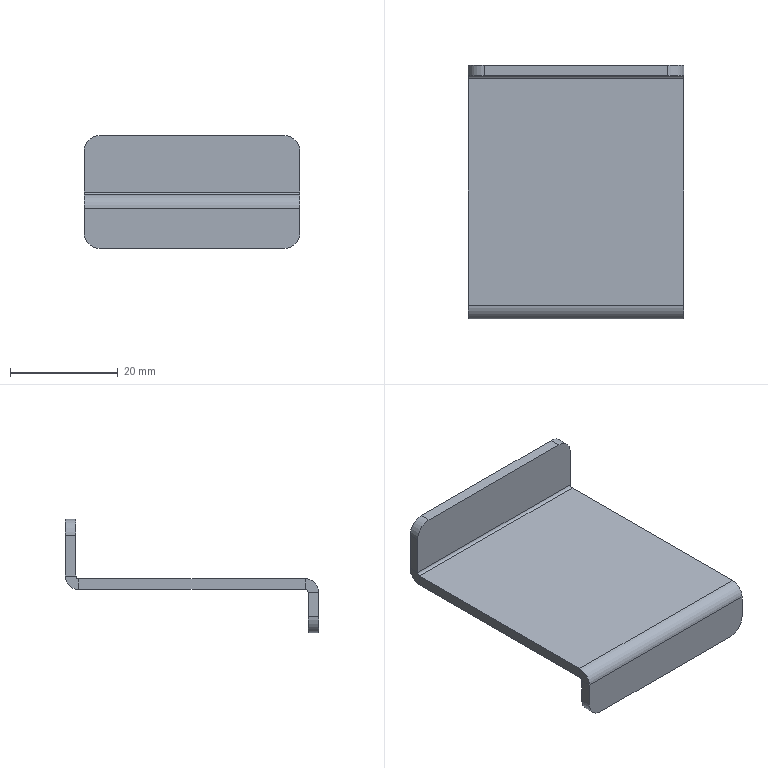Part | SolidWorks | features BaseBody 1 | 1 solid | 26 faces | box 40 x 47 x 21 mm | volume 5162 mm3 | plane 18 | cylinder 8 | commonest cylinder face diameters 6 x4 1 x2 5 x2
STEP:
#1=CARTESIAN_POINT('',(17.,-23.5,-10.));
#2=VERTEX_POINT('',#1);
#3=CARTESIAN_POINT('',(20.,-23.5,-7.));
#4=VERTEX_POINT('',#3);
#5=CARTESIAN_POINT('',(17.,-23.5,-7.));
#6=DIRECTION('',(0.,-1.,0.));
#7=DIRECTION('',(0.,0.,-1.));
#8=AXIS2_PLACEMENT_3D('',#5,#6,#7);
#9=CIRCLE('',#8,3.);
#10=EDGE_CURVE('',#2,#4,#9,.T.);
#11=ORIENTED_EDGE('',*,*,#10,.F.);
#12=CARTESIAN_POINT('',(17.,-21.5,-10.));
#13=VERTEX_POINT('',#12);
#14=CARTESIAN_POINT('',(17.,-23.5,-10.));
#15=DIRECTION('',(0.,-1.,0.));
#16=VECTOR('',#15,1000.);
#17=LINE('',#14,#16);
#18=EDGE_CURVE('',#13,#2,#17,.T.);
#19=ORIENTED_EDGE('',*,*,#18,.F.);
#20=CARTESIAN_POINT('',(20.,-21.5,-7.));
#21=VERTEX_POINT('',#20);
#22=CARTESIAN_POINT('',(17.,-21.5,-7.));
#23=DIRECTION('',(0.,1.,0.));
#24=DIRECTION('',(0.,0.,-1.));
#25=AXIS2_PLACEMENT_3D('',#22,#23,#24);
#26=CIRCLE('',#25,3.);
#27=EDGE_CURVE('',#21,#13,#26,.T.);
#28=ORIENTED_EDGE('',*,*,#27,.F.);
#29=CARTESIAN_POINT('',(20.,-23.5,-7.));
#30=DIRECTION('',(0.,1.,0.));
#31=VECTOR('',#30,1000.);
#32=LINE('',#29,#31);
#33=EDGE_CURVE('',#4,#21,#32,.T.);
#34=ORIENTED_EDGE('',*,*,#33,.F.);
#35=EDGE_LOOP('',(#11,#19,#28,#34));
#36=FACE_OUTER_BOUND('',#35,.T.);
#37=CARTESIAN_POINT('',(17.,-23.5,-7.));
#38=DIRECTION('',(0.,1.,0.));
#39=DIRECTION('',(0.,0.,1.));
#40=AXIS2_PLACEMENT_3D('',#37,#38,#39);
#41=CYLINDRICAL_SURFACE('',#40,3.);
#42=ADVANCED_FACE('',(#36),#41,.T.);
#43=CARTESIAN_POINT('',(-20.,-23.5,-7.));
#44=VERTEX_POINT('',#43);
#45=CARTESIAN_POINT('',(-17.,-23.5,-10.));
#46=VERTEX_POINT('',#45);
#47=CARTESIAN_POINT('',(-17.,-23.5,-7.));
#48=DIRECTION('',(0.,-1.,0.));
#49=DIRECTION('',(0.,0.,-1.));
#50=AXIS2_PLACEMENT_3D('',#47,#48,#49);
#51=CIRCLE('',#50,3.);
#52=EDGE_CURVE('',#44,#46,#51,.T.);
#53=ORIENTED_EDGE('',*,*,#52,.F.);
#54=CARTESIAN_POINT('',(-20.,-21.5,-7.));
#55=VERTEX_POINT('',#54);
#56=CARTESIAN_POINT('',(-20.,-23.5,-7.));
#57=DIRECTION('',(0.,-1.,0.));
#58=VECTOR('',#57,1000.);
#59=LINE('',#56,#58);
#60=EDGE_CURVE('',#55,#44,#59,.T.);
#61=ORIENTED_EDGE('',*,*,#60,.F.);
#62=CARTESIAN_POINT('',(-17.,-21.5,-10.));
#63=VERTEX_POINT('',#62);
#64=CARTESIAN_POINT('',(-17.,-21.5,-7.));
#65=DIRECTION('',(0.,1.,0.));
#66=DIRECTION('',(0.,0.,-1.));
#67=AXIS2_PLACEMENT_3D('',#64,#65,#66);
#68=CIRCLE('',#67,3.);
#69=EDGE_CURVE('',#63,#55,#68,.T.);
#70=ORIENTED_EDGE('',*,*,#69,.F.);
#71=CARTESIAN_POINT('',(-17.,-23.5,-10.));
#72=DIRECTION('',(0.,1.,0.));
#73=VECTOR('',#72,1000.);
#74=LINE('',#71,#73);
#75=EDGE_CURVE('',#46,#63,#74,.T.);
#76=ORIENTED_EDGE('',*,*,#75,.F.);
#77=EDGE_LOOP('',(#53,#61,#70,#76));
#78=FACE_OUTER_BOUND('',#77,.T.);
#79=CARTESIAN_POINT('',(-17.,-23.5,-7.));
#80=DIRECTION('',(0.,1.,0.));
#81=DIRECTION('',(0.,0.,1.));
#82=AXIS2_PLACEMENT_3D('',#79,#80,#81);
#83=CYLINDRICAL_SURFACE('',#82,3.);
#84=ADVANCED_FACE('',(#78),#83,.T.);
#85=CARTESIAN_POINT('',(17.,23.5,11.));
#86=VERTEX_POINT('',#85);
#87=CARTESIAN_POINT('',(20.,23.5,8.));
#88=VERTEX_POINT('',#87);
#89=CARTESIAN_POINT('',(17.,23.5,8.));
#90=DIRECTION('',(0.,1.,0.));
#91=DIRECTION('',(0.,0.,-1.));
#92=AXIS2_PLACEMENT_3D('',#89,#90,#91);
#93=CIRCLE('',#92,3.);
#94=EDGE_CURVE('',#86,#88,#93,.T.);
#95=ORIENTED_EDGE('',*,*,#94,.F.);
#96=CARTESIAN_POINT('',(17.,21.5,11.));
#97=VERTEX_POINT('',#96);
#98=CARTESIAN_POINT('',(17.,23.5,11.));
#99=DIRECTION('',(0.,1.,0.));
#100=VECTOR('',#99,1000.);
#101=LINE('',#98,#100);
#102=EDGE_CURVE('',#97,#86,#101,.T.);
#103=ORIENTED_EDGE('',*,*,#102,.F.);
#104=CARTESIAN_POINT('',(20.,21.5,8.));
#105=VERTEX_POINT('',#104);
#106=CARTESIAN_POINT('',(17.,21.5,8.));
#107=DIRECTION('',(0.,-1.,0.));
#108=DIRECTION('',(0.,0.,-1.));
#109=AXIS2_PLACEMENT_3D('',#106,#107,#108);
#110=CIRCLE('',#109,3.);
#111=EDGE_CURVE('',#105,#97,#110,.T.);
#112=ORIENTED_EDGE('',*,*,#111,.F.);
#113=CARTESIAN_POINT('',(20.,23.5,8.));
#114=DIRECTION('',(0.,-1.,0.));
#115=VECTOR('',#114,1000.);
#116=LINE('',#113,#115);
#117=EDGE_CURVE('',#88,#105,#116,.T.);
#118=ORIENTED_EDGE('',*,*,#117,.F.);
#119=EDGE_LOOP('',(#95,#103,#112,#118));
#120=FACE_OUTER_BOUND('',#119,.T.);
#121=CARTESIAN_POINT('',(17.,23.5,8.));
#122=DIRECTION('',(0.,-1.,0.));
#123=DIRECTION('',(0.,0.,-1.));
#124=AXIS2_PLACEMENT_3D('',#121,#122,#123);
#125=CYLINDRICAL_SURFACE('',#124,3.);
#126=ADVANCED_FACE('',(#120),#125,.T.);
#127=CARTESIAN_POINT('',(-20.,23.5,8.));
#128=VERTEX_POINT('',#127);
#129=CARTESIAN_POINT('',(-17.,23.5,11.));
#130=VERTEX_POINT('',#129);
#131=CARTESIAN_POINT('',(-17.,23.5,8.));
#132=DIRECTION('',(0.,1.,0.));
#133=DIRECTION('',(0.,0.,-1.));
#134=AXIS2_PLACEMENT_3D('',#131,#132,#133);
#135=CIRCLE('',#134,3.);
#136=EDGE_CURVE('',#128,#130,#135,.T.);
#137=ORIENTED_EDGE('',*,*,#136,.F.);
#138=CARTESIAN_POINT('',(-20.,21.5,8.));
#139=VERTEX_POINT('',#138);
#140=CARTESIAN_POINT('',(-20.,23.5,8.));
#141=DIRECTION('',(0.,1.,0.));
#142=VECTOR('',#141,1000.);
#143=LINE('',#140,#142);
#144=EDGE_CURVE('',#139,#128,#143,.T.);
#145=ORIENTED_EDGE('',*,*,#144,.F.);
#146=CARTESIAN_POINT('',(-17.,21.5,11.));
#147=VERTEX_POINT('',#146);
#148=CARTESIAN_POINT('',(-17.,21.5,8.));
#149=DIRECTION('',(0.,-1.,0.));
#150=DIRECTION('',(0.,0.,-1.));
#151=AXIS2_PLACEMENT_3D('',#148,#149,#150);
#152=CIRCLE('',#151,3.);
#153=EDGE_CURVE('',#147,#139,#152,.T.);
#154=ORIENTED_EDGE('',*,*,#153,.F.);
#155=CARTESIAN_POINT('',(-17.,23.5,11.));
#156=DIRECTION('',(0.,-1.,0.));
#157=VECTOR('',#156,1000.);
#158=LINE('',#155,#157);
#159=EDGE_CURVE('',#130,#147,#158,.T.);
#160=ORIENTED_EDGE('',*,*,#159,.F.);
#161=EDGE_LOOP('',(#137,#145,#154,#160));
#162=FACE_OUTER_BOUND('',#161,.T.);
#163=CARTESIAN_POINT('',(-17.,23.5,8.));
#164=DIRECTION('',(0.,-1.,0.));
#165=DIRECTION('',(0.,0.,-1.));
#166=AXIS2_PLACEMENT_3D('',#163,#164,#165);
#167=CYLINDRICAL_SURFACE('',#166,3.);
#168=ADVANCED_FACE('',(#162),#167,.T.);
#169=CARTESIAN_POINT('',(0.,23.5,11.));
#170=DIRECTION('',(1.,0.,0.));
#171=VECTOR('',#170,1000.);
#172=LINE('',#169,#171);
#173=EDGE_CURVE('',#130,#86,#172,.T.);
#174=ORIENTED_EDGE('',*,*,#173,.F.);
#175=ORIENTED_EDGE('',*,*,#159,.T.);
#176=CARTESIAN_POINT('',(20.,21.5,11.));
#177=DIRECTION('',(1.,0.,0.));
#178=VECTOR('',#177,1000.);
#179=LINE('',#176,#178);
#180=EDGE_CURVE('',#147,#97,#179,.T.);
#181=ORIENTED_EDGE('',*,*,#180,.T.);
#182=ORIENTED_EDGE('',*,*,#102,.T.);
#183=EDGE_LOOP('',(#174,#175,#181,#182));
#184=FACE_OUTER_BOUND('',#183,.T.);
#185=CARTESIAN_POINT('',(20.,23.5,11.));
#186=DIRECTION('',(0.,0.,-1.));
#187=DIRECTION('',(0.,-1.,0.));
#188=AXIS2_PLACEMENT_3D('',#185,#186,#187);
#189=PLANE('',#188);
#190=ADVANCED_FACE('',(#184),#189,.F.);
#191=ORIENTED_EDGE('',*,*,#180,.F.);
#192=ORIENTED_EDGE('',*,*,#153,.T.);
#193=CARTESIAN_POINT('',(-20.,21.5,0.5));
#194=VERTEX_POINT('',#193);
#195=CARTESIAN_POINT('',(-20.,21.5,11.));
#196=DIRECTION('',(0.,0.,1.));
#197=VECTOR('',#196,1000.);
#198=LINE('',#195,#197);
#199=EDGE_CURVE('',#194,#139,#198,.T.);
#200=ORIENTED_EDGE('',*,*,#199,.F.);
#201=CARTESIAN_POINT('',(20.,21.5,0.5));
#202=VERTEX_POINT('',#201);
#203=CARTESIAN_POINT('',(20.,21.5,0.5));
#204=DIRECTION('',(-1.,0.,0.));
#205=VECTOR('',#204,1000.);
#206=LINE('',#203,#205);
#207=EDGE_CURVE('',#202,#194,#206,.T.);
#208=ORIENTED_EDGE('',*,*,#207,.F.);
#209=CARTESIAN_POINT('',(20.,21.5,0.));
#210=DIRECTION('',(0.,0.,-1.));
#211=VECTOR('',#210,1000.);
#212=LINE('',#209,#211);
#213=EDGE_CURVE('',#105,#202,#212,.T.);
#214=ORIENTED_EDGE('',*,*,#213,.F.);
#215=ORIENTED_EDGE('',*,*,#111,.T.);
#216=EDGE_LOOP('',(#191,#192,#200,#208,#214,#215));
#217=FACE_OUTER_BOUND('',#216,.T.);
#218=CARTESIAN_POINT('',(0.,21.5,0.));
#219=DIRECTION('',(0.,-1.,0.));
#220=DIRECTION('',(-1.,0.,0.));
#221=AXIS2_PLACEMENT_3D('',#218,#219,#220);
#222=PLANE('',#221);
#223=ADVANCED_FACE('',(#217),#222,.T.);
#224=CARTESIAN_POINT('',(-20.,23.5,0.5));
#225=VERTEX_POINT('',#224);
#226=CARTESIAN_POINT('',(-20.,23.5,0.));
#227=DIRECTION('',(0.,0.,1.));
#228=VECTOR('',#227,1000.);
#229=LINE('',#226,#228);
#230=EDGE_CURVE('',#225,#128,#229,.T.);
#231=ORIENTED_EDGE('',*,*,#230,.T.);
#232=ORIENTED_EDGE('',*,*,#136,.T.);
#233=ORIENTED_EDGE('',*,*,#173,.T.);
#234=ORIENTED_EDGE('',*,*,#94,.T.);
#235=CARTESIAN_POINT('',(20.,23.5,0.5));
#236=VERTEX_POINT('',#235);
#237=CARTESIAN_POINT('',(20.,23.5,0.));
#238=DIRECTION('',(0.,0.,-1.));
#239=VECTOR('',#238,1000.);
#240=LINE('',#237,#239);
#241=EDGE_CURVE('',#88,#236,#240,.T.);
#242=ORIENTED_EDGE('',*,*,#241,.T.);
#243=CARTESIAN_POINT('',(20.,23.5,0.5));
#244=DIRECTION('',(1.,0.,0.));
#245=VECTOR('',#244,1000.);
#246=LINE('',#243,#245);
#247=EDGE_CURVE('',#225,#236,#246,.T.);
#248=ORIENTED_EDGE('',*,*,#247,.F.);
#249=EDGE_LOOP('',(#231,#232,#233,#234,#242,#248));
#250=FACE_OUTER_BOUND('',#249,.T.);
#251=CARTESIAN_POINT('',(0.,23.5,0.));
#252=DIRECTION('',(0.,-1.,0.));
#253=DIRECTION('',(-1.,0.,0.));
#254=AXIS2_PLACEMENT_3D('',#251,#252,#253);
#255=PLANE('',#254);
#256=ADVANCED_FACE('',(#250),#255,.F.);
#257=ORIENTED_EDGE('',*,*,#199,.T.);
#258=ORIENTED_EDGE('',*,*,#144,.T.);
#259=ORIENTED_EDGE('',*,*,#230,.F.);
#260=CARTESIAN_POINT('',(-20.,21.5,0.5));
#261=DIRECTION('',(0.,1.,0.));
#262=VECTOR('',#261,1000.);
#263=LINE('',#260,#262);
#264=EDGE_CURVE('',#194,#225,#263,.T.);
#265=ORIENTED_EDGE('',*,*,#264,.F.);
#266=EDGE_LOOP('',(#257,#258,#259,#265));
#267=FACE_OUTER_BOUND('',#266,.T.);
#268=CARTESIAN_POINT('',(-20.,23.5,11.));
#269=DIRECTION('',(1.,0.,0.));
#270=DIRECTION('',(0.,1.,0.));
#271=AXIS2_PLACEMENT_3D('',#268,#269,#270);
#272=PLANE('',#271);
#273=ADVANCED_FACE('',(#267),#272,.F.);
#274=ORIENTED_EDGE('',*,*,#241,.F.);
#275=ORIENTED_EDGE('',*,*,#117,.T.);
#276=ORIENTED_EDGE('',*,*,#213,.T.);
#277=CARTESIAN_POINT('',(20.,23.5,0.5));
#278=DIRECTION('',(0.,1.,0.));
#279=VECTOR('',#278,1000.);
#280=LINE('',#277,#279);
#281=EDGE_CURVE('',#202,#236,#280,.T.);
#282=ORIENTED_EDGE('',*,*,#281,.T.);
#283=EDGE_LOOP('',(#274,#275,#276,#282));
#284=FACE_OUTER_BOUND('',#283,.T.);
#285=CARTESIAN_POINT('',(20.,23.5,0.));
#286=DIRECTION('',(-1.,0.,0.));
#287=DIRECTION('',(0.,0.,1.));
#288=AXIS2_PLACEMENT_3D('',#285,#286,#287);
#289=PLANE('',#288);
#290=ADVANCED_FACE('',(#284),#289,.F.);
#291=CARTESIAN_POINT('',(-20.,21.,0.));
#292=VERTEX_POINT('',#291);
#293=CARTESIAN_POINT('',(20.,21.,0.));
#294=VERTEX_POINT('',#293);
#295=CARTESIAN_POINT('',(-20.,21.,0.));
#296=DIRECTION('',(1.,0.,0.));
#297=VECTOR('',#296,1000.);
#298=LINE('',#295,#297);
#299=EDGE_CURVE('',#292,#294,#298,.T.);
#300=ORIENTED_EDGE('',*,*,#299,.T.);
#301=CARTESIAN_POINT('',(20.,21.,0.5));
#302=DIRECTION('',(1.,0.,0.));
#303=DIRECTION('',(0.,0.,1.));
#304=AXIS2_PLACEMENT_3D('',#301,#302,#303);
#305=CIRCLE('',#304,0.5);
#306=EDGE_CURVE('',#294,#202,#305,.T.);
#307=ORIENTED_EDGE('',*,*,#306,.T.);
#308=ORIENTED_EDGE('',*,*,#207,.T.);
#309=CARTESIAN_POINT('',(-20.,21.,0.5));
#310=DIRECTION('',(-1.,0.,0.));
#311=DIRECTION('',(0.,0.,1.));
#312=AXIS2_PLACEMENT_3D('',#309,#310,#311);
#313=CIRCLE('',#312,0.5);
#314=EDGE_CURVE('',#194,#292,#313,.T.);
#315=ORIENTED_EDGE('',*,*,#314,.T.);
#316=EDGE_LOOP('',(#300,#307,#308,#315));
#317=FACE_OUTER_BOUND('',#316,.T.);
#318=CARTESIAN_POINT('',(-20.,21.,0.5));
#319=DIRECTION('',(-1.,0.,0.));
#320=DIRECTION('',(0.,1.,0.));
#321=AXIS2_PLACEMENT_3D('',#318,#319,#320);
#322=CYLINDRICAL_SURFACE('',#321,0.5);
#323=ADVANCED_FACE('',(#317),#322,.F.);
#324=CARTESIAN_POINT('',(-20.,21.,-2.));
#325=VERTEX_POINT('',#324);
#326=CARTESIAN_POINT('',(20.,21.,-2.));
#327=VERTEX_POINT('',#326);
#328=CARTESIAN_POINT('',(-20.,21.,-2.));
#329=DIRECTION('',(1.,0.,0.));
#330=VECTOR('',#329,1000.);
#331=LINE('',#328,#330);
#332=EDGE_CURVE('',#325,#327,#331,.T.);
#333=ORIENTED_EDGE('',*,*,#332,.F.);
#334=CARTESIAN_POINT('',(-20.,21.,0.5));
#335=DIRECTION('',(-1.,0.,0.));
#336=DIRECTION('',(0.,0.,1.));
#337=AXIS2_PLACEMENT_3D('',#334,#335,#336);
#338=CIRCLE('',#337,2.5);
#339=EDGE_CURVE('',#225,#325,#338,.T.);
#340=ORIENTED_EDGE('',*,*,#339,.F.);
#341=ORIENTED_EDGE('',*,*,#247,.T.);
#342=CARTESIAN_POINT('',(20.,21.,0.5));
#343=DIRECTION('',(1.,0.,0.));
#344=DIRECTION('',(0.,0.,1.));
#345=AXIS2_PLACEMENT_3D('',#342,#343,#344);
#346=CIRCLE('',#345,2.5);
#347=EDGE_CURVE('',#327,#236,#346,.T.);
#348=ORIENTED_EDGE('',*,*,#347,.F.);
#349=EDGE_LOOP('',(#333,#340,#341,#348));
#350=FACE_OUTER_BOUND('',#349,.T.);
#351=CARTESIAN_POINT('',(-20.,21.,0.5));
#352=DIRECTION('',(-1.,0.,0.));
#353=DIRECTION('',(0.,1.,0.));
#354=AXIS2_PLACEMENT_3D('',#351,#352,#353);
#355=CYLINDRICAL_SURFACE('',#354,2.5);
#356=ADVANCED_FACE('',(#350),#355,.T.);
#357=ORIENTED_EDGE('',*,*,#314,.F.);
#358=ORIENTED_EDGE('',*,*,#264,.T.);
#359=ORIENTED_EDGE('',*,*,#339,.T.);
#360=CARTESIAN_POINT('',(-20.,21.,0.));
#361=DIRECTION('',(0.,0.,-1.));
#362=VECTOR('',#361,1000.);
#363=LINE('',#360,#362);
#364=EDGE_CURVE('',#292,#325,#363,.T.);
#365=ORIENTED_EDGE('',*,*,#364,.F.);
#366=EDGE_LOOP('',(#357,#358,#359,#365));
#367=FACE_OUTER_BOUND('',#366,.T.);
#368=CARTESIAN_POINT('',(-20.,21.,0.5));
#369=DIRECTION('',(1.,0.,0.));
#370=DIRECTION('',(0.,0.,-1.));
#371=AXIS2_PLACEMENT_3D('',#368,#369,#370);
#372=PLANE('',#371);
#373=ADVANCED_FACE('',(#367),#372,.F.);
#374=ORIENTED_EDGE('',*,*,#281,.F.);
#375=ORIENTED_EDGE('',*,*,#306,.F.);
#376=CARTESIAN_POINT('',(20.,21.,0.));
#377=DIRECTION('',(0.,0.,-1.));
#378=VECTOR('',#377,1000.);
#379=LINE('',#376,#378);
#380=EDGE_CURVE('',#294,#327,#379,.T.);
#381=ORIENTED_EDGE('',*,*,#380,.T.);
#382=ORIENTED_EDGE('',*,*,#347,.T.);
#383=EDGE_LOOP('',(#374,#375,#381,#382));
#384=FACE_OUTER_BOUND('',#383,.T.);
#385=CARTESIAN_POINT('',(20.,21.,0.5));
#386=DIRECTION('',(1.,0.,0.));
#387=DIRECTION('',(0.,0.,-1.));
#388=AXIS2_PLACEMENT_3D('',#385,#386,#387);
#389=PLANE('',#388);
#390=ADVANCED_FACE('',(#384),#389,.T.);
#391=CARTESIAN_POINT('',(-20.,-23.5,-10.));
#392=DIRECTION('',(-1.,0.,0.));
#393=VECTOR('',#392,1000.);
#394=LINE('',#391,#393);
#395=EDGE_CURVE('',#2,#46,#394,.T.);
#396=ORIENTED_EDGE('',*,*,#395,.T.);
#397=ORIENTED_EDGE('',*,*,#75,.T.);
#398=CARTESIAN_POINT('',(0.,-21.5,-10.));
#399=DIRECTION('',(-1.,0.,0.));
#400=VECTOR('',#399,1000.);
#401=LINE('',#398,#400);
#402=EDGE_CURVE('',#13,#63,#401,.T.);
#403=ORIENTED_EDGE('',*,*,#402,.F.);
#404=ORIENTED_EDGE('',*,*,#18,.T.);
#405=EDGE_LOOP('',(#396,#397,#403,#404));
#406=FACE_OUTER_BOUND('',#405,.T.);
#407=CARTESIAN_POINT('',(-20.,-23.5,-10.));
#408=DIRECTION('',(0.,0.,-1.));
#409=DIRECTION('',(0.,-1.,0.));
#410=AXIS2_PLACEMENT_3D('',#407,#408,#409);
#411=PLANE('',#410);
#412=ADVANCED_FACE('',(#406),#411,.T.);
#413=ORIENTED_EDGE('',*,*,#402,.T.);
#414=ORIENTED_EDGE('',*,*,#69,.T.);
#415=CARTESIAN_POINT('',(-20.,-21.5,-2.5));
#416=VERTEX_POINT('',#415);
#417=CARTESIAN_POINT('',(-20.,-21.5,0.));
#418=DIRECTION('',(0.,0.,1.));
#419=VECTOR('',#418,1000.);
#420=LINE('',#417,#419);
#421=EDGE_CURVE('',#55,#416,#420,.T.);
#422=ORIENTED_EDGE('',*,*,#421,.T.);
#423=CARTESIAN_POINT('',(20.,-21.5,-2.5));
#424=VERTEX_POINT('',#423);
#425=CARTESIAN_POINT('',(20.,-21.5,-2.5));
#426=DIRECTION('',(-1.,0.,0.));
#427=VECTOR('',#426,1000.);
#428=LINE('',#425,#427);
#429=EDGE_CURVE('',#424,#416,#428,.T.);
#430=ORIENTED_EDGE('',*,*,#429,.F.);
#431=CARTESIAN_POINT('',(20.,-21.5,0.));
#432=DIRECTION('',(0.,0.,-1.));
#433=VECTOR('',#432,1000.);
#434=LINE('',#431,#433);
#435=EDGE_CURVE('',#424,#21,#434,.T.);
#436=ORIENTED_EDGE('',*,*,#435,.T.);
#437=ORIENTED_EDGE('',*,*,#27,.T.);
#438=EDGE_LOOP('',(#413,#414,#422,#430,#436,#437));
#439=FACE_OUTER_BOUND('',#438,.T.);
#440=CARTESIAN_POINT('',(0.,-21.5,0.));
#441=DIRECTION('',(0.,-1.,0.));
#442=DIRECTION('',(-1.,0.,0.));
#443=AXIS2_PLACEMENT_3D('',#440,#441,#442);
#444=PLANE('',#443);
#445=ADVANCED_FACE('',(#439),#444,.F.);
#446=CARTESIAN_POINT('',(-20.,-23.5,-2.5));
#447=VERTEX_POINT('',#446);
#448=CARTESIAN_POINT('',(-20.,-23.5,-2.));
#449=DIRECTION('',(0.,0.,1.));
#450=VECTOR('',#449,1000.);
#451=LINE('',#448,#450);
#452=EDGE_CURVE('',#44,#447,#451,.T.);
#453=ORIENTED_EDGE('',*,*,#452,.F.);
#454=ORIENTED_EDGE('',*,*,#52,.T.);
#455=ORIENTED_EDGE('',*,*,#395,.F.);
#456=ORIENTED_EDGE('',*,*,#10,.T.);
#457=CARTESIAN_POINT('',(20.,-23.5,-2.5));
#458=VERTEX_POINT('',#457);
#459=CARTESIAN_POINT('',(20.,-23.5,-10.));
#460=DIRECTION('',(0.,0.,-1.));
#461=VECTOR('',#460,1000.);
#462=LINE('',#459,#461);
#463=EDGE_CURVE('',#458,#4,#462,.T.);
#464=ORIENTED_EDGE('',*,*,#463,.F.);
#465=CARTESIAN_POINT('',(0.,-23.5,-2.5));
#466=DIRECTION('',(-1.,0.,0.));
#467=VECTOR('',#466,1000.);
#468=LINE('',#465,#467);
#469=EDGE_CURVE('',#458,#447,#468,.T.);
#470=ORIENTED_EDGE('',*,*,#469,.T.);
#471=EDGE_LOOP('',(#453,#454,#455,#456,#464,#470));
#472=FACE_OUTER_BOUND('',#471,.T.);
#473=CARTESIAN_POINT('',(0.,-23.5,0.));
#474=DIRECTION('',(0.,-1.,0.));
#475=DIRECTION('',(-1.,0.,0.));
#476=AXIS2_PLACEMENT_3D('',#473,#474,#475);
#477=PLANE('',#476);
#478=ADVANCED_FACE('',(#472),#477,.T.);
#479=ORIENTED_EDGE('',*,*,#463,.T.);
#480=ORIENTED_EDGE('',*,*,#33,.T.);
#481=ORIENTED_EDGE('',*,*,#435,.F.);
#482=CARTESIAN_POINT('',(20.,-23.5,-2.5));
#483=DIRECTION('',(0.,-1.,0.));
#484=VECTOR('',#483,1000.);
#485=LINE('',#482,#484);
#486=EDGE_CURVE('',#424,#458,#485,.T.);
#487=ORIENTED_EDGE('',*,*,#486,.T.);
#488=EDGE_LOOP('',(#479,#480,#481,#487));
#489=FACE_OUTER_BOUND('',#488,.T.);
#490=CARTESIAN_POINT('',(20.,-23.5,-10.));
#491=DIRECTION('',(1.,0.,0.));
#492=DIRECTION('',(0.,0.,-1.));
#493=AXIS2_PLACEMENT_3D('',#490,#491,#492);
#494=PLANE('',#493);
#495=ADVANCED_FACE('',(#489),#494,.T.);
#496=ORIENTED_EDGE('',*,*,#421,.F.);
#497=ORIENTED_EDGE('',*,*,#60,.T.);
#498=ORIENTED_EDGE('',*,*,#452,.T.);
#499=CARTESIAN_POINT('',(-20.,-21.5,-2.5));
#500=DIRECTION('',(0.,-1.,0.));
#501=VECTOR('',#500,1000.);
#502=LINE('',#499,#501);
#503=EDGE_CURVE('',#416,#447,#502,.T.);
#504=ORIENTED_EDGE('',*,*,#503,.F.);
#505=EDGE_LOOP('',(#496,#497,#498,#504));
#506=FACE_OUTER_BOUND('',#505,.T.);
#507=CARTESIAN_POINT('',(-20.,-23.5,-2.));
#508=DIRECTION('',(-1.,0.,0.));
#509=DIRECTION('',(0.,0.,1.));
#510=AXIS2_PLACEMENT_3D('',#507,#508,#509);
#511=PLANE('',#510);
#512=ADVANCED_FACE('',(#506),#511,.T.);
#513=CARTESIAN_POINT('',(-20.,-21.,-2.));
#514=VERTEX_POINT('',#513);
#515=CARTESIAN_POINT('',(20.,-21.,-2.));
#516=VERTEX_POINT('',#515);
#517=CARTESIAN_POINT('',(-20.,-21.,-2.));
#518=DIRECTION('',(1.,0.,0.));
#519=VECTOR('',#518,1000.);
#520=LINE('',#517,#519);
#521=EDGE_CURVE('',#514,#516,#520,.T.);
#522=ORIENTED_EDGE('',*,*,#521,.T.);
#523=CARTESIAN_POINT('',(20.,-21.,-2.5));
#524=DIRECTION('',(1.,0.,0.));
#525=DIRECTION('',(0.,0.,1.));
#526=AXIS2_PLACEMENT_3D('',#523,#524,#525);
#527=CIRCLE('',#526,0.5);
#528=EDGE_CURVE('',#516,#424,#527,.T.);
#529=ORIENTED_EDGE('',*,*,#528,.T.);
#530=ORIENTED_EDGE('',*,*,#429,.T.);
#531=CARTESIAN_POINT('',(-20.,-21.,-2.5));
#532=DIRECTION('',(-1.,0.,0.));
#533=DIRECTION('',(0.,0.,1.));
#534=AXIS2_PLACEMENT_3D('',#531,#532,#533);
#535=CIRCLE('',#534,0.5);
#536=EDGE_CURVE('',#416,#514,#535,.T.);
#537=ORIENTED_EDGE('',*,*,#536,.T.);
#538=EDGE_LOOP('',(#522,#529,#530,#537));
#539=FACE_OUTER_BOUND('',#538,.T.);
#540=CARTESIAN_POINT('',(-20.,-21.,-2.5));
#541=DIRECTION('',(-1.,0.,0.));
#542=DIRECTION('',(0.,-1.,0.));
#543=AXIS2_PLACEMENT_3D('',#540,#541,#542);
#544=CYLINDRICAL_SURFACE('',#543,0.5);
#545=ADVANCED_FACE('',(#539),#544,.F.);
#546=CARTESIAN_POINT('',(-20.,-21.,0.));
#547=VERTEX_POINT('',#546);
#548=CARTESIAN_POINT('',(20.,-21.,0.));
#549=VERTEX_POINT('',#548);
#550=CARTESIAN_POINT('',(-20.,-21.,0.));
#551=DIRECTION('',(1.,0.,0.));
#552=VECTOR('',#551,1000.);
#553=LINE('',#550,#552);
#554=EDGE_CURVE('',#547,#549,#553,.T.);
#555=ORIENTED_EDGE('',*,*,#554,.F.);
#556=CARTESIAN_POINT('',(-20.,-21.,-2.5));
#557=DIRECTION('',(-1.,0.,0.));
#558=DIRECTION('',(0.,0.,1.));
#559=AXIS2_PLACEMENT_3D('',#556,#557,#558);
#560=CIRCLE('',#559,2.5);
#561=EDGE_CURVE('',#447,#547,#560,.T.);
#562=ORIENTED_EDGE('',*,*,#561,.F.);
#563=ORIENTED_EDGE('',*,*,#469,.F.);
#564=CARTESIAN_POINT('',(20.,-21.,-2.5));
#565=DIRECTION('',(1.,0.,0.));
#566=DIRECTION('',(0.,0.,1.));
#567=AXIS2_PLACEMENT_3D('',#564,#565,#566);
#568=CIRCLE('',#567,2.5);
#569=EDGE_CURVE('',#549,#458,#568,.T.);
#570=ORIENTED_EDGE('',*,*,#569,.F.);
#571=EDGE_LOOP('',(#555,#562,#563,#570));
#572=FACE_OUTER_BOUND('',#571,.T.);
#573=CARTESIAN_POINT('',(-20.,-21.,-2.5));
#574=DIRECTION('',(-1.,0.,0.));
#575=DIRECTION('',(0.,-1.,0.));
#576=AXIS2_PLACEMENT_3D('',#573,#574,#575);
#577=CYLINDRICAL_SURFACE('',#576,2.5);
#578=ADVANCED_FACE('',(#572),#577,.T.);
#579=ORIENTED_EDGE('',*,*,#536,.F.);
#580=ORIENTED_EDGE('',*,*,#503,.T.);
#581=ORIENTED_EDGE('',*,*,#561,.T.);
#582=CARTESIAN_POINT('',(-20.,-21.,-2.));
#583=DIRECTION('',(0.,0.,1.));
#584=VECTOR('',#583,1000.);
#585=LINE('',#582,#584);
#586=EDGE_CURVE('',#514,#547,#585,.T.);
#587=ORIENTED_EDGE('',*,*,#586,.F.);
#588=EDGE_LOOP('',(#579,#580,#581,#587));
#589=FACE_OUTER_BOUND('',#588,.T.);
#590=CARTESIAN_POINT('',(-20.,-21.,-2.5));
#591=DIRECTION('',(1.,0.,0.));
#592=DIRECTION('',(0.,1.,0.));
#593=AXIS2_PLACEMENT_3D('',#590,#591,#592);
#594=PLANE('',#593);
#595=ADVANCED_FACE('',(#589),#594,.F.);
#596=ORIENTED_EDGE('',*,*,#486,.F.);
#597=ORIENTED_EDGE('',*,*,#528,.F.);
#598=CARTESIAN_POINT('',(20.,-21.,-2.));
#599=DIRECTION('',(0.,0.,1.));
#600=VECTOR('',#599,1000.);
#601=LINE('',#598,#600);
#602=EDGE_CURVE('',#516,#549,#601,.T.);
#603=ORIENTED_EDGE('',*,*,#602,.T.);
#604=ORIENTED_EDGE('',*,*,#569,.T.);
#605=EDGE_LOOP('',(#596,#597,#603,#604));
#606=FACE_OUTER_BOUND('',#605,.T.);
#607=CARTESIAN_POINT('',(20.,-21.,-2.5));
#608=DIRECTION('',(1.,0.,0.));
#609=DIRECTION('',(0.,1.,0.));
#610=AXIS2_PLACEMENT_3D('',#607,#608,#609);
#611=PLANE('',#610);
#612=ADVANCED_FACE('',(#606),#611,.T.);
#613=ORIENTED_EDGE('',*,*,#380,.F.);
#614=CARTESIAN_POINT('',(20.,23.5,0.));
#615=DIRECTION('',(0.,1.,0.));
#616=VECTOR('',#615,1000.);
#617=LINE('',#614,#616);
#618=EDGE_CURVE('',#549,#294,#617,.T.);
#619=ORIENTED_EDGE('',*,*,#618,.F.);
#620=ORIENTED_EDGE('',*,*,#602,.F.);
#621=CARTESIAN_POINT('',(20.,23.5,-2.));
#622=DIRECTION('',(0.,1.,0.));
#623=VECTOR('',#622,1000.);
#624=LINE('',#621,#623);
#625=EDGE_CURVE('',#516,#327,#624,.T.);
#626=ORIENTED_EDGE('',*,*,#625,.T.);
#627=EDGE_LOOP('',(#613,#619,#620,#626));
#628=FACE_OUTER_BOUND('',#627,.T.);
#629=CARTESIAN_POINT('',(20.,23.5,-2.));
#630=DIRECTION('',(1.,0.,0.));
#631=DIRECTION('',(0.,1.,0.));
#632=AXIS2_PLACEMENT_3D('',#629,#630,#631);
#633=PLANE('',#632);
#634=ADVANCED_FACE('',(#628),#633,.T.);
#635=ORIENTED_EDGE('',*,*,#618,.T.);
#636=ORIENTED_EDGE('',*,*,#299,.F.);
#637=CARTESIAN_POINT('',(-20.,23.5,0.));
#638=DIRECTION('',(0.,-1.,0.));
#639=VECTOR('',#638,1000.);
#640=LINE('',#637,#639);
#641=EDGE_CURVE('',#292,#547,#640,.T.);
#642=ORIENTED_EDGE('',*,*,#641,.T.);
#643=ORIENTED_EDGE('',*,*,#554,.T.);
#644=EDGE_LOOP('',(#635,#636,#642,#643));
#645=FACE_OUTER_BOUND('',#644,.T.);
#646=CARTESIAN_POINT('',(0.,0.,0.));
#647=DIRECTION('',(0.,0.,1.));
#648=DIRECTION('',(1.,0.,0.));
#649=AXIS2_PLACEMENT_3D('',#646,#647,#648);
#650=PLANE('',#649);
#651=ADVANCED_FACE('',(#645),#650,.T.);
#652=ORIENTED_EDGE('',*,*,#332,.T.);
#653=ORIENTED_EDGE('',*,*,#625,.F.);
#654=ORIENTED_EDGE('',*,*,#521,.F.);
#655=CARTESIAN_POINT('',(-20.,23.5,-2.));
#656=DIRECTION('',(0.,-1.,0.));
#657=VECTOR('',#656,1000.);
#658=LINE('',#655,#657);
#659=EDGE_CURVE('',#325,#514,#658,.T.);
#660=ORIENTED_EDGE('',*,*,#659,.F.);
#661=EDGE_LOOP('',(#652,#653,#654,#660));
#662=FACE_OUTER_BOUND('',#661,.T.);
#663=CARTESIAN_POINT('',(0.,0.,-2.));
#664=DIRECTION('',(0.,0.,1.));
#665=DIRECTION('',(1.,0.,0.));
#666=AXIS2_PLACEMENT_3D('',#663,#664,#665);
#667=PLANE('',#666);
#668=ADVANCED_FACE('',(#662),#667,.F.);
#669=ORIENTED_EDGE('',*,*,#641,.F.);
#670=ORIENTED_EDGE('',*,*,#364,.T.);
#671=ORIENTED_EDGE('',*,*,#659,.T.);
#672=ORIENTED_EDGE('',*,*,#586,.T.);
#673=EDGE_LOOP('',(#669,#670,#671,#672));
#674=FACE_OUTER_BOUND('',#673,.T.);
#675=CARTESIAN_POINT('',(-20.,23.5,-2.));
#676=DIRECTION('',(-1.,0.,0.));
#677=DIRECTION('',(0.,1.,0.));
#678=AXIS2_PLACEMENT_3D('',#675,#676,#677);
#679=PLANE('',#678);
#680=ADVANCED_FACE('',(#674),#679,.T.);
#681=CLOSED_SHELL('',(#42,#84,#126,#168,#190,#223,#256,#273,#290,#323,#356,#373,#390,#412,#445,#478,#495,#512,#545,#578,#595,#612,#634,#651,#668,#680));
#682=MANIFOLD_SOLID_BREP('',#681);
#683=CARTESIAN_POINT('',(0.,0.,0.));
#684=DIRECTION('',(0.,0.,1.));
#685=DIRECTION('',(1.,0.,0.));
#686=AXIS2_PLACEMENT_3D('',#683,#684,#685);
#687=(LENGTH_UNIT()NAMED_UNIT(*)SI_UNIT(.MILLI.,.METRE.));
#688=UNCERTAINTY_MEASURE_WITH_UNIT(LENGTH_MEASURE(0.00001),#687,'','');
#689=(NAMED_UNIT(*)PLANE_ANGLE_UNIT()SI_UNIT($,.RADIAN.));
#690=(NAMED_UNIT(*)SI_UNIT($,.STERADIAN.)SOLID_ANGLE_UNIT());
#691=(GEOMETRIC_REPRESENTATION_CONTEXT(3)GLOBAL_UNCERTAINTY_ASSIGNED_CONTEXT((#688))GLOBAL_UNIT_ASSIGNED_CONTEXT((#687,#689,#690))REPRESENTATION_CONTEXT('',''));
#692=ADVANCED_BREP_SHAPE_REPRESENTATION('',(#682,#686),#691);